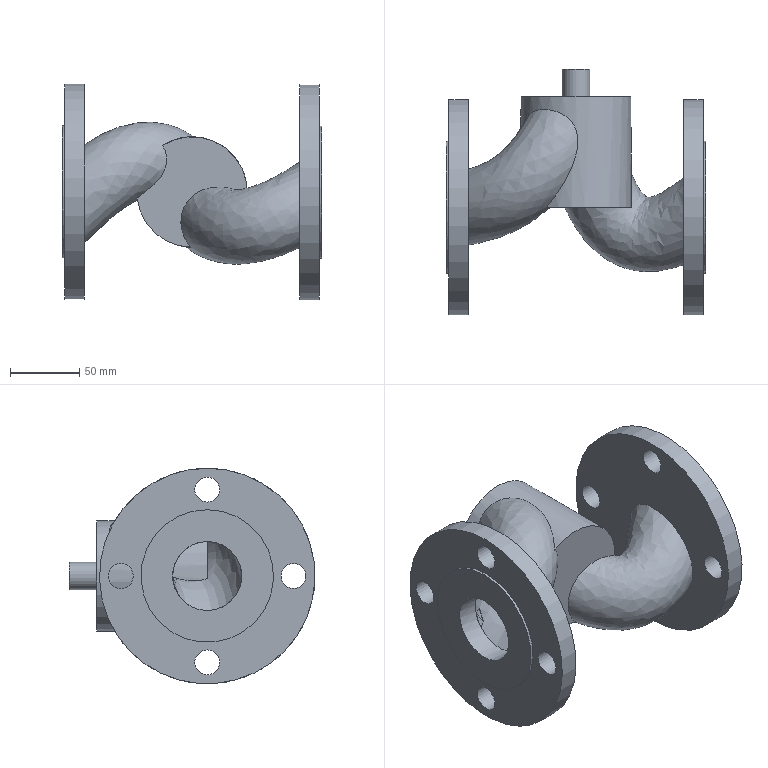Part | STEP file | Part 11 | 1 solid | 44 faces | box 188 x 178 x 156 mm | volume 934142 mm3 | cylinder 21 | plane 18 | spline 5 | commonest cylinder face diameters 18 x8 50 x4 80 x3 96 x2 156 x2 20 x1